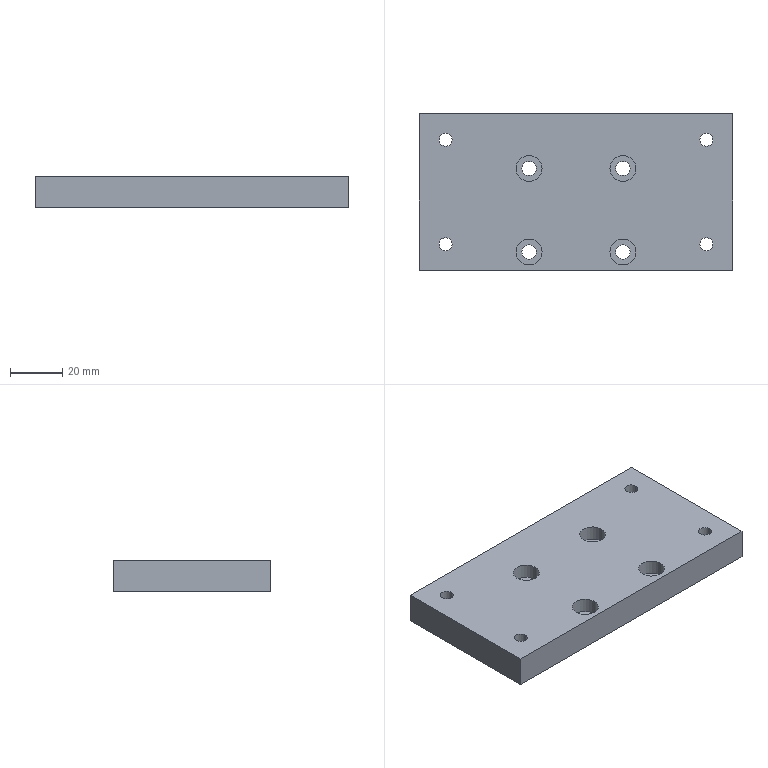Part | SolidWorks | features HoleWzd 2, 3DProfileFeature 1, Extrusion 1 | 1 solid | 34 faces | box 120 x 60 x 12 mm | volume 83068 mm3 | cylinder 24 | plane 10 | commonest cylinder face diameters 5 x8 5.5 x8 10 x8
STEP:
#1=CARTESIAN_POINT('',(-47.5,20.,0.));
#2=VERTEX_POINT('',#1);
#3=CARTESIAN_POINT('',(-52.5,20.,0.));
#4=VERTEX_POINT('',#3);
#5=CARTESIAN_POINT('',(-50.,20.,0.));
#6=DIRECTION('',(0.,0.,-1.));
#7=DIRECTION('',(-1.,0.,0.));
#8=AXIS2_PLACEMENT_3D('',#5,#6,#7);
#9=CIRCLE('',#8,2.5);
#10=EDGE_CURVE('',#2,#4,#9,.T.);
#11=ORIENTED_EDGE('',*,*,#10,.T.);
#12=CARTESIAN_POINT('',(-52.5,20.,12.));
#13=VERTEX_POINT('',#12);
#14=CARTESIAN_POINT('',(-52.5,20.,12.));
#15=DIRECTION('',(0.,0.,1.));
#16=VECTOR('',#15,1000.);
#17=LINE('',#14,#16);
#18=EDGE_CURVE('',#4,#13,#17,.T.);
#19=ORIENTED_EDGE('',*,*,#18,.T.);
#20=CARTESIAN_POINT('',(-47.5,20.,12.));
#21=VERTEX_POINT('',#20);
#22=CARTESIAN_POINT('',(-50.,20.,12.));
#23=DIRECTION('',(0.,0.,1.));
#24=DIRECTION('',(1.,0.,0.));
#25=AXIS2_PLACEMENT_3D('',#22,#23,#24);
#26=CIRCLE('',#25,2.5);
#27=EDGE_CURVE('',#13,#21,#26,.T.);
#28=ORIENTED_EDGE('',*,*,#27,.T.);
#29=CARTESIAN_POINT('',(-47.5,20.,12.));
#30=DIRECTION('',(0.,0.,1.));
#31=VECTOR('',#30,1000.);
#32=LINE('',#29,#31);
#33=EDGE_CURVE('',#2,#21,#32,.T.);
#34=ORIENTED_EDGE('',*,*,#33,.F.);
#35=EDGE_LOOP('',(#11,#19,#28,#34));
#36=FACE_OUTER_BOUND('',#35,.T.);
#37=CARTESIAN_POINT('',(-50.,20.,12.));
#38=DIRECTION('',(0.,0.,1.));
#39=DIRECTION('',(1.,0.,0.));
#40=AXIS2_PLACEMENT_3D('',#37,#38,#39);
#41=CYLINDRICAL_SURFACE('',#40,2.5);
#42=ADVANCED_FACE('',(#36),#41,.F.);
#43=CARTESIAN_POINT('',(-47.5,-20.,0.));
#44=VERTEX_POINT('',#43);
#45=CARTESIAN_POINT('',(-52.5,-20.,0.));
#46=VERTEX_POINT('',#45);
#47=CARTESIAN_POINT('',(-50.,-20.,0.));
#48=DIRECTION('',(0.,0.,-1.));
#49=DIRECTION('',(-1.,0.,0.));
#50=AXIS2_PLACEMENT_3D('',#47,#48,#49);
#51=CIRCLE('',#50,2.5);
#52=EDGE_CURVE('',#44,#46,#51,.T.);
#53=ORIENTED_EDGE('',*,*,#52,.T.);
#54=CARTESIAN_POINT('',(-52.5,-20.,12.));
#55=VERTEX_POINT('',#54);
#56=CARTESIAN_POINT('',(-52.5,-20.,12.));
#57=DIRECTION('',(0.,0.,1.));
#58=VECTOR('',#57,1000.);
#59=LINE('',#56,#58);
#60=EDGE_CURVE('',#46,#55,#59,.T.);
#61=ORIENTED_EDGE('',*,*,#60,.T.);
#62=CARTESIAN_POINT('',(-47.5,-20.,12.));
#63=VERTEX_POINT('',#62);
#64=CARTESIAN_POINT('',(-50.,-20.,12.));
#65=DIRECTION('',(0.,0.,1.));
#66=DIRECTION('',(1.,0.,0.));
#67=AXIS2_PLACEMENT_3D('',#64,#65,#66);
#68=CIRCLE('',#67,2.5);
#69=EDGE_CURVE('',#55,#63,#68,.T.);
#70=ORIENTED_EDGE('',*,*,#69,.T.);
#71=CARTESIAN_POINT('',(-47.5,-20.,12.));
#72=DIRECTION('',(0.,0.,1.));
#73=VECTOR('',#72,1000.);
#74=LINE('',#71,#73);
#75=EDGE_CURVE('',#44,#63,#74,.T.);
#76=ORIENTED_EDGE('',*,*,#75,.F.);
#77=EDGE_LOOP('',(#53,#61,#70,#76));
#78=FACE_OUTER_BOUND('',#77,.T.);
#79=CARTESIAN_POINT('',(-50.,-20.,12.));
#80=DIRECTION('',(0.,0.,1.));
#81=DIRECTION('',(1.,0.,0.));
#82=AXIS2_PLACEMENT_3D('',#79,#80,#81);
#83=CYLINDRICAL_SURFACE('',#82,2.5);
#84=ADVANCED_FACE('',(#78),#83,.F.);
#85=CARTESIAN_POINT('',(52.5,-20.,0.));
#86=VERTEX_POINT('',#85);
#87=CARTESIAN_POINT('',(47.5,-20.,0.));
#88=VERTEX_POINT('',#87);
#89=CARTESIAN_POINT('',(50.,-20.,0.));
#90=DIRECTION('',(0.,0.,-1.));
#91=DIRECTION('',(-1.,0.,0.));
#92=AXIS2_PLACEMENT_3D('',#89,#90,#91);
#93=CIRCLE('',#92,2.5);
#94=EDGE_CURVE('',#86,#88,#93,.T.);
#95=ORIENTED_EDGE('',*,*,#94,.T.);
#96=CARTESIAN_POINT('',(47.5,-20.,12.));
#97=VERTEX_POINT('',#96);
#98=CARTESIAN_POINT('',(47.5,-20.,12.));
#99=DIRECTION('',(0.,0.,1.));
#100=VECTOR('',#99,1000.);
#101=LINE('',#98,#100);
#102=EDGE_CURVE('',#88,#97,#101,.T.);
#103=ORIENTED_EDGE('',*,*,#102,.T.);
#104=CARTESIAN_POINT('',(52.5,-20.,12.));
#105=VERTEX_POINT('',#104);
#106=CARTESIAN_POINT('',(50.,-20.,12.));
#107=DIRECTION('',(0.,0.,1.));
#108=DIRECTION('',(1.,0.,0.));
#109=AXIS2_PLACEMENT_3D('',#106,#107,#108);
#110=CIRCLE('',#109,2.5);
#111=EDGE_CURVE('',#97,#105,#110,.T.);
#112=ORIENTED_EDGE('',*,*,#111,.T.);
#113=CARTESIAN_POINT('',(52.5,-20.,12.));
#114=DIRECTION('',(0.,0.,1.));
#115=VECTOR('',#114,1000.);
#116=LINE('',#113,#115);
#117=EDGE_CURVE('',#86,#105,#116,.T.);
#118=ORIENTED_EDGE('',*,*,#117,.F.);
#119=EDGE_LOOP('',(#95,#103,#112,#118));
#120=FACE_OUTER_BOUND('',#119,.T.);
#121=CARTESIAN_POINT('',(50.,-20.,12.));
#122=DIRECTION('',(0.,0.,1.));
#123=DIRECTION('',(1.,0.,0.));
#124=AXIS2_PLACEMENT_3D('',#121,#122,#123);
#125=CYLINDRICAL_SURFACE('',#124,2.5);
#126=ADVANCED_FACE('',(#120),#125,.F.);
#127=CARTESIAN_POINT('',(52.5,20.,0.));
#128=VERTEX_POINT('',#127);
#129=CARTESIAN_POINT('',(47.5,20.,0.));
#130=VERTEX_POINT('',#129);
#131=CARTESIAN_POINT('',(50.,20.,0.));
#132=DIRECTION('',(0.,0.,-1.));
#133=DIRECTION('',(-1.,0.,0.));
#134=AXIS2_PLACEMENT_3D('',#131,#132,#133);
#135=CIRCLE('',#134,2.5);
#136=EDGE_CURVE('',#128,#130,#135,.T.);
#137=ORIENTED_EDGE('',*,*,#136,.T.);
#138=CARTESIAN_POINT('',(47.5,20.,12.));
#139=VERTEX_POINT('',#138);
#140=CARTESIAN_POINT('',(47.5,20.,12.));
#141=DIRECTION('',(0.,0.,1.));
#142=VECTOR('',#141,1000.);
#143=LINE('',#140,#142);
#144=EDGE_CURVE('',#130,#139,#143,.T.);
#145=ORIENTED_EDGE('',*,*,#144,.T.);
#146=CARTESIAN_POINT('',(52.5,20.,12.));
#147=VERTEX_POINT('',#146);
#148=CARTESIAN_POINT('',(50.,20.,12.));
#149=DIRECTION('',(0.,0.,1.));
#150=DIRECTION('',(1.,0.,0.));
#151=AXIS2_PLACEMENT_3D('',#148,#149,#150);
#152=CIRCLE('',#151,2.5);
#153=EDGE_CURVE('',#139,#147,#152,.T.);
#154=ORIENTED_EDGE('',*,*,#153,.T.);
#155=CARTESIAN_POINT('',(52.5,20.,12.));
#156=DIRECTION('',(0.,0.,1.));
#157=VECTOR('',#156,1000.);
#158=LINE('',#155,#157);
#159=EDGE_CURVE('',#128,#147,#158,.T.);
#160=ORIENTED_EDGE('',*,*,#159,.F.);
#161=EDGE_LOOP('',(#137,#145,#154,#160));
#162=FACE_OUTER_BOUND('',#161,.T.);
#163=CARTESIAN_POINT('',(50.,20.,12.));
#164=DIRECTION('',(0.,0.,1.));
#165=DIRECTION('',(1.,0.,0.));
#166=AXIS2_PLACEMENT_3D('',#163,#164,#165);
#167=CYLINDRICAL_SURFACE('',#166,2.5);
#168=ADVANCED_FACE('',(#162),#167,.F.);
#169=CARTESIAN_POINT('',(-23.,9.,6.3));
#170=VERTEX_POINT('',#169);
#171=CARTESIAN_POINT('',(-13.,9.,6.3));
#172=VERTEX_POINT('',#171);
#173=CARTESIAN_POINT('',(-18.,9.,6.3));
#174=DIRECTION('',(0.,0.,1.));
#175=DIRECTION('',(1.,0.,0.));
#176=AXIS2_PLACEMENT_3D('',#173,#174,#175);
#177=CIRCLE('',#176,5.);
#178=EDGE_CURVE('',#170,#172,#177,.T.);
#179=ORIENTED_EDGE('',*,*,#178,.F.);
#180=CARTESIAN_POINT('',(-23.,9.,12.));
#181=VERTEX_POINT('',#180);
#182=CARTESIAN_POINT('',(-23.,9.,12.));
#183=DIRECTION('',(0.,0.,1.));
#184=VECTOR('',#183,1000.);
#185=LINE('',#182,#184);
#186=EDGE_CURVE('',#170,#181,#185,.T.);
#187=ORIENTED_EDGE('',*,*,#186,.T.);
#188=CARTESIAN_POINT('',(-13.,9.,12.));
#189=VERTEX_POINT('',#188);
#190=CARTESIAN_POINT('',(-18.,9.,12.));
#191=DIRECTION('',(0.,0.,1.));
#192=DIRECTION('',(1.,0.,0.));
#193=AXIS2_PLACEMENT_3D('',#190,#191,#192);
#194=CIRCLE('',#193,5.);
#195=EDGE_CURVE('',#181,#189,#194,.T.);
#196=ORIENTED_EDGE('',*,*,#195,.T.);
#197=CARTESIAN_POINT('',(-13.,9.,12.));
#198=DIRECTION('',(0.,0.,1.));
#199=VECTOR('',#198,1000.);
#200=LINE('',#197,#199);
#201=EDGE_CURVE('',#172,#189,#200,.T.);
#202=ORIENTED_EDGE('',*,*,#201,.F.);
#203=EDGE_LOOP('',(#179,#187,#196,#202));
#204=FACE_OUTER_BOUND('',#203,.T.);
#205=CARTESIAN_POINT('',(-18.,9.,12.));
#206=DIRECTION('',(0.,0.,1.));
#207=DIRECTION('',(1.,0.,0.));
#208=AXIS2_PLACEMENT_3D('',#205,#206,#207);
#209=CYLINDRICAL_SURFACE('',#208,5.);
#210=ADVANCED_FACE('',(#204),#209,.F.);
#211=CARTESIAN_POINT('',(-15.25,9.,0.));
#212=VERTEX_POINT('',#211);
#213=CARTESIAN_POINT('',(-20.75,9.,0.));
#214=VERTEX_POINT('',#213);
#215=CARTESIAN_POINT('',(-18.,9.,0.));
#216=DIRECTION('',(0.,0.,-1.));
#217=DIRECTION('',(-1.,0.,0.));
#218=AXIS2_PLACEMENT_3D('',#215,#216,#217);
#219=CIRCLE('',#218,2.75);
#220=EDGE_CURVE('',#212,#214,#219,.T.);
#221=ORIENTED_EDGE('',*,*,#220,.T.);
#222=CARTESIAN_POINT('',(-20.75,9.,6.3));
#223=VERTEX_POINT('',#222);
#224=CARTESIAN_POINT('',(-20.75,9.,12.));
#225=DIRECTION('',(0.,0.,1.));
#226=VECTOR('',#225,1000.);
#227=LINE('',#224,#226);
#228=EDGE_CURVE('',#214,#223,#227,.T.);
#229=ORIENTED_EDGE('',*,*,#228,.T.);
#230=CARTESIAN_POINT('',(-15.25,9.,6.3));
#231=VERTEX_POINT('',#230);
#232=CARTESIAN_POINT('',(-18.,9.,6.3));
#233=DIRECTION('',(0.,0.,1.));
#234=DIRECTION('',(1.,0.,0.));
#235=AXIS2_PLACEMENT_3D('',#232,#233,#234);
#236=CIRCLE('',#235,2.75);
#237=EDGE_CURVE('',#223,#231,#236,.T.);
#238=ORIENTED_EDGE('',*,*,#237,.T.);
#239=CARTESIAN_POINT('',(-15.25,9.,12.));
#240=DIRECTION('',(0.,0.,1.));
#241=VECTOR('',#240,1000.);
#242=LINE('',#239,#241);
#243=EDGE_CURVE('',#212,#231,#242,.T.);
#244=ORIENTED_EDGE('',*,*,#243,.F.);
#245=EDGE_LOOP('',(#221,#229,#238,#244));
#246=FACE_OUTER_BOUND('',#245,.T.);
#247=CARTESIAN_POINT('',(-18.,9.,12.));
#248=DIRECTION('',(0.,0.,1.));
#249=DIRECTION('',(1.,0.,0.));
#250=AXIS2_PLACEMENT_3D('',#247,#248,#249);
#251=CYLINDRICAL_SURFACE('',#250,2.75);
#252=ADVANCED_FACE('',(#246),#251,.F.);
#253=CARTESIAN_POINT('',(13.,9.,6.3));
#254=VERTEX_POINT('',#253);
#255=CARTESIAN_POINT('',(23.,9.,6.3));
#256=VERTEX_POINT('',#255);
#257=CARTESIAN_POINT('',(18.,9.,6.3));
#258=DIRECTION('',(0.,0.,1.));
#259=DIRECTION('',(1.,0.,0.));
#260=AXIS2_PLACEMENT_3D('',#257,#258,#259);
#261=CIRCLE('',#260,5.);
#262=EDGE_CURVE('',#254,#256,#261,.T.);
#263=ORIENTED_EDGE('',*,*,#262,.F.);
#264=CARTESIAN_POINT('',(13.,9.,12.));
#265=VERTEX_POINT('',#264);
#266=CARTESIAN_POINT('',(13.,9.,12.));
#267=DIRECTION('',(0.,0.,1.));
#268=VECTOR('',#267,1000.);
#269=LINE('',#266,#268);
#270=EDGE_CURVE('',#254,#265,#269,.T.);
#271=ORIENTED_EDGE('',*,*,#270,.T.);
#272=CARTESIAN_POINT('',(23.,9.,12.));
#273=VERTEX_POINT('',#272);
#274=CARTESIAN_POINT('',(18.,9.,12.));
#275=DIRECTION('',(0.,0.,1.));
#276=DIRECTION('',(1.,0.,0.));
#277=AXIS2_PLACEMENT_3D('',#274,#275,#276);
#278=CIRCLE('',#277,5.);
#279=EDGE_CURVE('',#265,#273,#278,.T.);
#280=ORIENTED_EDGE('',*,*,#279,.T.);
#281=CARTESIAN_POINT('',(23.,9.,12.));
#282=DIRECTION('',(0.,0.,1.));
#283=VECTOR('',#282,1000.);
#284=LINE('',#281,#283);
#285=EDGE_CURVE('',#256,#273,#284,.T.);
#286=ORIENTED_EDGE('',*,*,#285,.F.);
#287=EDGE_LOOP('',(#263,#271,#280,#286));
#288=FACE_OUTER_BOUND('',#287,.T.);
#289=CARTESIAN_POINT('',(18.,9.,12.));
#290=DIRECTION('',(0.,0.,1.));
#291=DIRECTION('',(1.,0.,0.));
#292=AXIS2_PLACEMENT_3D('',#289,#290,#291);
#293=CYLINDRICAL_SURFACE('',#292,5.);
#294=ADVANCED_FACE('',(#288),#293,.F.);
#295=CARTESIAN_POINT('',(20.75,9.,0.));
#296=VERTEX_POINT('',#295);
#297=CARTESIAN_POINT('',(15.25,9.,0.));
#298=VERTEX_POINT('',#297);
#299=CARTESIAN_POINT('',(18.,9.,0.));
#300=DIRECTION('',(0.,0.,-1.));
#301=DIRECTION('',(-1.,0.,0.));
#302=AXIS2_PLACEMENT_3D('',#299,#300,#301);
#303=CIRCLE('',#302,2.75);
#304=EDGE_CURVE('',#296,#298,#303,.T.);
#305=ORIENTED_EDGE('',*,*,#304,.T.);
#306=CARTESIAN_POINT('',(15.25,9.,6.3));
#307=VERTEX_POINT('',#306);
#308=CARTESIAN_POINT('',(15.25,9.,12.));
#309=DIRECTION('',(0.,0.,1.));
#310=VECTOR('',#309,1000.);
#311=LINE('',#308,#310);
#312=EDGE_CURVE('',#298,#307,#311,.T.);
#313=ORIENTED_EDGE('',*,*,#312,.T.);
#314=CARTESIAN_POINT('',(20.75,9.,6.3));
#315=VERTEX_POINT('',#314);
#316=CARTESIAN_POINT('',(18.,9.,6.3));
#317=DIRECTION('',(0.,0.,1.));
#318=DIRECTION('',(1.,0.,0.));
#319=AXIS2_PLACEMENT_3D('',#316,#317,#318);
#320=CIRCLE('',#319,2.75);
#321=EDGE_CURVE('',#307,#315,#320,.T.);
#322=ORIENTED_EDGE('',*,*,#321,.T.);
#323=CARTESIAN_POINT('',(20.75,9.,12.));
#324=DIRECTION('',(0.,0.,1.));
#325=VECTOR('',#324,1000.);
#326=LINE('',#323,#325);
#327=EDGE_CURVE('',#296,#315,#326,.T.);
#328=ORIENTED_EDGE('',*,*,#327,.F.);
#329=EDGE_LOOP('',(#305,#313,#322,#328));
#330=FACE_OUTER_BOUND('',#329,.T.);
#331=CARTESIAN_POINT('',(18.,9.,12.));
#332=DIRECTION('',(0.,0.,1.));
#333=DIRECTION('',(1.,0.,0.));
#334=AXIS2_PLACEMENT_3D('',#331,#332,#333);
#335=CYLINDRICAL_SURFACE('',#334,2.75);
#336=ADVANCED_FACE('',(#330),#335,.F.);
#337=CARTESIAN_POINT('',(-23.,-23.,6.3));
#338=VERTEX_POINT('',#337);
#339=CARTESIAN_POINT('',(-13.,-23.,6.3));
#340=VERTEX_POINT('',#339);
#341=CARTESIAN_POINT('',(-18.,-23.,6.3));
#342=DIRECTION('',(0.,0.,1.));
#343=DIRECTION('',(1.,0.,0.));
#344=AXIS2_PLACEMENT_3D('',#341,#342,#343);
#345=CIRCLE('',#344,5.);
#346=EDGE_CURVE('',#338,#340,#345,.T.);
#347=ORIENTED_EDGE('',*,*,#346,.F.);
#348=CARTESIAN_POINT('',(-23.,-23.,12.));
#349=VERTEX_POINT('',#348);
#350=CARTESIAN_POINT('',(-23.,-23.,12.));
#351=DIRECTION('',(0.,0.,1.));
#352=VECTOR('',#351,1000.);
#353=LINE('',#350,#352);
#354=EDGE_CURVE('',#338,#349,#353,.T.);
#355=ORIENTED_EDGE('',*,*,#354,.T.);
#356=CARTESIAN_POINT('',(-13.,-23.,12.));
#357=VERTEX_POINT('',#356);
#358=CARTESIAN_POINT('',(-18.,-23.,12.));
#359=DIRECTION('',(0.,0.,1.));
#360=DIRECTION('',(1.,0.,0.));
#361=AXIS2_PLACEMENT_3D('',#358,#359,#360);
#362=CIRCLE('',#361,5.);
#363=EDGE_CURVE('',#349,#357,#362,.T.);
#364=ORIENTED_EDGE('',*,*,#363,.T.);
#365=CARTESIAN_POINT('',(-13.,-23.,12.));
#366=DIRECTION('',(0.,0.,1.));
#367=VECTOR('',#366,1000.);
#368=LINE('',#365,#367);
#369=EDGE_CURVE('',#340,#357,#368,.T.);
#370=ORIENTED_EDGE('',*,*,#369,.F.);
#371=EDGE_LOOP('',(#347,#355,#364,#370));
#372=FACE_OUTER_BOUND('',#371,.T.);
#373=CARTESIAN_POINT('',(-18.,-23.,12.));
#374=DIRECTION('',(0.,0.,1.));
#375=DIRECTION('',(1.,0.,0.));
#376=AXIS2_PLACEMENT_3D('',#373,#374,#375);
#377=CYLINDRICAL_SURFACE('',#376,5.);
#378=ADVANCED_FACE('',(#372),#377,.F.);
#379=CARTESIAN_POINT('',(-15.25,-23.,0.));
#380=VERTEX_POINT('',#379);
#381=CARTESIAN_POINT('',(-20.75,-23.,0.));
#382=VERTEX_POINT('',#381);
#383=CARTESIAN_POINT('',(-18.,-23.,0.));
#384=DIRECTION('',(0.,0.,-1.));
#385=DIRECTION('',(-1.,0.,0.));
#386=AXIS2_PLACEMENT_3D('',#383,#384,#385);
#387=CIRCLE('',#386,2.75);
#388=EDGE_CURVE('',#380,#382,#387,.T.);
#389=ORIENTED_EDGE('',*,*,#388,.T.);
#390=CARTESIAN_POINT('',(-20.75,-23.,6.3));
#391=VERTEX_POINT('',#390);
#392=CARTESIAN_POINT('',(-20.75,-23.,12.));
#393=DIRECTION('',(0.,0.,1.));
#394=VECTOR('',#393,1000.);
#395=LINE('',#392,#394);
#396=EDGE_CURVE('',#382,#391,#395,.T.);
#397=ORIENTED_EDGE('',*,*,#396,.T.);
#398=CARTESIAN_POINT('',(-15.25,-23.,6.3));
#399=VERTEX_POINT('',#398);
#400=CARTESIAN_POINT('',(-18.,-23.,6.3));
#401=DIRECTION('',(0.,0.,1.));
#402=DIRECTION('',(1.,0.,0.));
#403=AXIS2_PLACEMENT_3D('',#400,#401,#402);
#404=CIRCLE('',#403,2.75);
#405=EDGE_CURVE('',#391,#399,#404,.T.);
#406=ORIENTED_EDGE('',*,*,#405,.T.);
#407=CARTESIAN_POINT('',(-15.25,-23.,12.));
#408=DIRECTION('',(0.,0.,1.));
#409=VECTOR('',#408,1000.);
#410=LINE('',#407,#409);
#411=EDGE_CURVE('',#380,#399,#410,.T.);
#412=ORIENTED_EDGE('',*,*,#411,.F.);
#413=EDGE_LOOP('',(#389,#397,#406,#412));
#414=FACE_OUTER_BOUND('',#413,.T.);
#415=CARTESIAN_POINT('',(-18.,-23.,12.));
#416=DIRECTION('',(0.,0.,1.));
#417=DIRECTION('',(1.,0.,0.));
#418=AXIS2_PLACEMENT_3D('',#415,#416,#417);
#419=CYLINDRICAL_SURFACE('',#418,2.75);
#420=ADVANCED_FACE('',(#414),#419,.F.);
#421=CARTESIAN_POINT('',(13.,-23.,6.3));
#422=VERTEX_POINT('',#421);
#423=CARTESIAN_POINT('',(23.,-23.,6.3));
#424=VERTEX_POINT('',#423);
#425=CARTESIAN_POINT('',(18.,-23.,6.3));
#426=DIRECTION('',(0.,0.,1.));
#427=DIRECTION('',(1.,0.,0.));
#428=AXIS2_PLACEMENT_3D('',#425,#426,#427);
#429=CIRCLE('',#428,5.);
#430=EDGE_CURVE('',#422,#424,#429,.T.);
#431=ORIENTED_EDGE('',*,*,#430,.F.);
#432=CARTESIAN_POINT('',(13.,-23.,12.));
#433=VERTEX_POINT('',#432);
#434=CARTESIAN_POINT('',(13.,-23.,12.));
#435=DIRECTION('',(0.,0.,1.));
#436=VECTOR('',#435,1000.);
#437=LINE('',#434,#436);
#438=EDGE_CURVE('',#422,#433,#437,.T.);
#439=ORIENTED_EDGE('',*,*,#438,.T.);
#440=CARTESIAN_POINT('',(23.,-23.,12.));
#441=VERTEX_POINT('',#440);
#442=CARTESIAN_POINT('',(18.,-23.,12.));
#443=DIRECTION('',(0.,0.,1.));
#444=DIRECTION('',(1.,0.,0.));
#445=AXIS2_PLACEMENT_3D('',#442,#443,#444);
#446=CIRCLE('',#445,5.);
#447=EDGE_CURVE('',#433,#441,#446,.T.);
#448=ORIENTED_EDGE('',*,*,#447,.T.);
#449=CARTESIAN_POINT('',(23.,-23.,12.));
#450=DIRECTION('',(0.,0.,1.));
#451=VECTOR('',#450,1000.);
#452=LINE('',#449,#451);
#453=EDGE_CURVE('',#424,#441,#452,.T.);
#454=ORIENTED_EDGE('',*,*,#453,.F.);
#455=EDGE_LOOP('',(#431,#439,#448,#454));
#456=FACE_OUTER_BOUND('',#455,.T.);
#457=CARTESIAN_POINT('',(18.,-23.,12.));
#458=DIRECTION('',(0.,0.,1.));
#459=DIRECTION('',(1.,0.,0.));
#460=AXIS2_PLACEMENT_3D('',#457,#458,#459);
#461=CYLINDRICAL_SURFACE('',#460,5.);
#462=ADVANCED_FACE('',(#456),#461,.F.);
#463=CARTESIAN_POINT('',(20.75,-23.,0.));
#464=VERTEX_POINT('',#463);
#465=CARTESIAN_POINT('',(15.25,-23.,0.));
#466=VERTEX_POINT('',#465);
#467=CARTESIAN_POINT('',(18.,-23.,0.));
#468=DIRECTION('',(0.,0.,-1.));
#469=DIRECTION('',(-1.,0.,0.));
#470=AXIS2_PLACEMENT_3D('',#467,#468,#469);
#471=CIRCLE('',#470,2.75);
#472=EDGE_CURVE('',#464,#466,#471,.T.);
#473=ORIENTED_EDGE('',*,*,#472,.T.);
#474=CARTESIAN_POINT('',(15.25,-23.,6.3));
#475=VERTEX_POINT('',#474);
#476=CARTESIAN_POINT('',(15.25,-23.,12.));
#477=DIRECTION('',(0.,0.,1.));
#478=VECTOR('',#477,1000.);
#479=LINE('',#476,#478);
#480=EDGE_CURVE('',#466,#475,#479,.T.);
#481=ORIENTED_EDGE('',*,*,#480,.T.);
#482=CARTESIAN_POINT('',(20.75,-23.,6.3));
#483=VERTEX_POINT('',#482);
#484=CARTESIAN_POINT('',(18.,-23.,6.3));
#485=DIRECTION('',(0.,0.,1.));
#486=DIRECTION('',(1.,0.,0.));
#487=AXIS2_PLACEMENT_3D('',#484,#485,#486);
#488=CIRCLE('',#487,2.75);
#489=EDGE_CURVE('',#475,#483,#488,.T.);
#490=ORIENTED_EDGE('',*,*,#489,.T.);
#491=CARTESIAN_POINT('',(20.75,-23.,12.));
#492=DIRECTION('',(0.,0.,1.));
#493=VECTOR('',#492,1000.);
#494=LINE('',#491,#493);
#495=EDGE_CURVE('',#464,#483,#494,.T.);
#496=ORIENTED_EDGE('',*,*,#495,.F.);
#497=EDGE_LOOP('',(#473,#481,#490,#496));
#498=FACE_OUTER_BOUND('',#497,.T.);
#499=CARTESIAN_POINT('',(18.,-23.,12.));
#500=DIRECTION('',(0.,0.,1.));
#501=DIRECTION('',(1.,0.,0.));
#502=AXIS2_PLACEMENT_3D('',#499,#500,#501);
#503=CYLINDRICAL_SURFACE('',#502,2.75);
#504=ADVANCED_FACE('',(#498),#503,.F.);
#505=CARTESIAN_POINT('',(-50.,20.,12.));
#506=DIRECTION('',(0.,0.,1.));
#507=DIRECTION('',(1.,0.,0.));
#508=AXIS2_PLACEMENT_3D('',#505,#506,#507);
#509=CIRCLE('',#508,2.5);
#510=EDGE_CURVE('',#21,#13,#509,.T.);
#511=ORIENTED_EDGE('',*,*,#510,.F.);
#512=ORIENTED_EDGE('',*,*,#27,.F.);
#513=EDGE_LOOP('',(#511,#512));
#514=FACE_BOUND('',#513,.T.);
#515=CARTESIAN_POINT('',(-50.,-20.,12.));
#516=DIRECTION('',(0.,0.,1.));
#517=DIRECTION('',(1.,0.,0.));
#518=AXIS2_PLACEMENT_3D('',#515,#516,#517);
#519=CIRCLE('',#518,2.5);
#520=EDGE_CURVE('',#63,#55,#519,.T.);
#521=ORIENTED_EDGE('',*,*,#520,.F.);
#522=ORIENTED_EDGE('',*,*,#69,.F.);
#523=EDGE_LOOP('',(#521,#522));
#524=FACE_BOUND('',#523,.T.);
#525=CARTESIAN_POINT('',(50.,-20.,12.));
#526=DIRECTION('',(0.,0.,1.));
#527=DIRECTION('',(1.,0.,0.));
#528=AXIS2_PLACEMENT_3D('',#525,#526,#527);
#529=CIRCLE('',#528,2.5);
#530=EDGE_CURVE('',#105,#97,#529,.T.);
#531=ORIENTED_EDGE('',*,*,#530,.F.);
#532=ORIENTED_EDGE('',*,*,#111,.F.);
#533=EDGE_LOOP('',(#531,#532));
#534=FACE_BOUND('',#533,.T.);
#535=CARTESIAN_POINT('',(50.,20.,12.));
#536=DIRECTION('',(0.,0.,1.));
#537=DIRECTION('',(1.,0.,0.));
#538=AXIS2_PLACEMENT_3D('',#535,#536,#537);
#539=CIRCLE('',#538,2.5);
#540=EDGE_CURVE('',#147,#139,#539,.T.);
#541=ORIENTED_EDGE('',*,*,#540,.F.);
#542=ORIENTED_EDGE('',*,*,#153,.F.);
#543=EDGE_LOOP('',(#541,#542));
#544=FACE_BOUND('',#543,.T.);
#545=CARTESIAN_POINT('',(-18.,9.,12.));
#546=DIRECTION('',(0.,0.,1.));
#547=DIRECTION('',(1.,0.,0.));
#548=AXIS2_PLACEMENT_3D('',#545,#546,#547);
#549=CIRCLE('',#548,5.);
#550=EDGE_CURVE('',#189,#181,#549,.T.);
#551=ORIENTED_EDGE('',*,*,#550,.F.);
#552=ORIENTED_EDGE('',*,*,#195,.F.);
#553=EDGE_LOOP('',(#551,#552));
#554=FACE_BOUND('',#553,.T.);
#555=CARTESIAN_POINT('',(18.,9.,12.));
#556=DIRECTION('',(0.,0.,1.));
#557=DIRECTION('',(1.,0.,0.));
#558=AXIS2_PLACEMENT_3D('',#555,#556,#557);
#559=CIRCLE('',#558,5.);
#560=EDGE_CURVE('',#273,#265,#559,.T.);
#561=ORIENTED_EDGE('',*,*,#560,.F.);
#562=ORIENTED_EDGE('',*,*,#279,.F.);
#563=EDGE_LOOP('',(#561,#562));
#564=FACE_BOUND('',#563,.T.);
#565=CARTESIAN_POINT('',(-18.,-23.,12.));
#566=DIRECTION('',(0.,0.,1.));
#567=DIRECTION('',(1.,0.,0.));
#568=AXIS2_PLACEMENT_3D('',#565,#566,#567);
#569=CIRCLE('',#568,5.);
#570=EDGE_CURVE('',#357,#349,#569,.T.);
#571=ORIENTED_EDGE('',*,*,#570,.F.);
#572=ORIENTED_EDGE('',*,*,#363,.F.);
#573=EDGE_LOOP('',(#571,#572));
#574=FACE_BOUND('',#573,.T.);
#575=CARTESIAN_POINT('',(18.,-23.,12.));
#576=DIRECTION('',(0.,0.,1.));
#577=DIRECTION('',(1.,0.,0.));
#578=AXIS2_PLACEMENT_3D('',#575,#576,#577);
#579=CIRCLE('',#578,5.);
#580=EDGE_CURVE('',#441,#433,#579,.T.);
#581=ORIENTED_EDGE('',*,*,#580,.F.);
#582=ORIENTED_EDGE('',*,*,#447,.F.);
#583=EDGE_LOOP('',(#581,#582));
#584=FACE_BOUND('',#583,.T.);
#585=CARTESIAN_POINT('',(60.,-30.,12.));
#586=VERTEX_POINT('',#585);
#587=CARTESIAN_POINT('',(60.,30.,12.));
#588=VERTEX_POINT('',#587);
#589=CARTESIAN_POINT('',(60.,-30.,12.));
#590=DIRECTION('',(0.,1.,0.));
#591=VECTOR('',#590,1000.);
#592=LINE('',#589,#591);
#593=EDGE_CURVE('',#586,#588,#592,.T.);
#594=ORIENTED_EDGE('',*,*,#593,.T.);
#595=CARTESIAN_POINT('',(-60.,30.,12.));
#596=VERTEX_POINT('',#595);
#597=CARTESIAN_POINT('',(-60.,30.,12.));
#598=DIRECTION('',(-1.,0.,0.));
#599=VECTOR('',#598,1000.);
#600=LINE('',#597,#599);
#601=EDGE_CURVE('',#588,#596,#600,.T.);
#602=ORIENTED_EDGE('',*,*,#601,.T.);
#603=CARTESIAN_POINT('',(-60.,-30.,12.));
#604=VERTEX_POINT('',#603);
#605=CARTESIAN_POINT('',(-60.,-30.,12.));
#606=DIRECTION('',(0.,-1.,0.));
#607=VECTOR('',#606,1000.);
#608=LINE('',#605,#607);
#609=EDGE_CURVE('',#596,#604,#608,.T.);
#610=ORIENTED_EDGE('',*,*,#609,.T.);
#611=CARTESIAN_POINT('',(-60.,-30.,12.));
#612=DIRECTION('',(1.,0.,0.));
#613=VECTOR('',#612,1000.);
#614=LINE('',#611,#613);
#615=EDGE_CURVE('',#604,#586,#614,.T.);
#616=ORIENTED_EDGE('',*,*,#615,.T.);
#617=EDGE_LOOP('',(#594,#602,#610,#616));
#618=FACE_OUTER_BOUND('',#617,.T.);
#619=CARTESIAN_POINT('',(0.,0.,12.));
#620=DIRECTION('',(0.,0.,-1.));
#621=DIRECTION('',(-1.,0.,0.));
#622=AXIS2_PLACEMENT_3D('',#619,#620,#621);
#623=PLANE('',#622);
#624=ADVANCED_FACE('',(#514,#524,#534,#544,#554,#564,#574,#584,#618),#623,.F.);
#625=ORIENTED_EDGE('',*,*,#10,.F.);
#626=CARTESIAN_POINT('',(-50.,20.,0.));
#627=DIRECTION('',(0.,0.,-1.));
#628=DIRECTION('',(-1.,0.,0.));
#629=AXIS2_PLACEMENT_3D('',#626,#627,#628);
#630=CIRCLE('',#629,2.5);
#631=EDGE_CURVE('',#4,#2,#630,.T.);
#632=ORIENTED_EDGE('',*,*,#631,.F.);
#633=EDGE_LOOP('',(#625,#632));
#634=FACE_BOUND('',#633,.T.);
#635=ORIENTED_EDGE('',*,*,#52,.F.);
#636=CARTESIAN_POINT('',(-50.,-20.,0.));
#637=DIRECTION('',(0.,0.,-1.));
#638=DIRECTION('',(-1.,0.,0.));
#639=AXIS2_PLACEMENT_3D('',#636,#637,#638);
#640=CIRCLE('',#639,2.5);
#641=EDGE_CURVE('',#46,#44,#640,.T.);
#642=ORIENTED_EDGE('',*,*,#641,.F.);
#643=EDGE_LOOP('',(#635,#642));
#644=FACE_BOUND('',#643,.T.);
#645=ORIENTED_EDGE('',*,*,#94,.F.);
#646=CARTESIAN_POINT('',(50.,-20.,0.));
#647=DIRECTION('',(0.,0.,-1.));
#648=DIRECTION('',(-1.,0.,0.));
#649=AXIS2_PLACEMENT_3D('',#646,#647,#648);
#650=CIRCLE('',#649,2.5);
#651=EDGE_CURVE('',#88,#86,#650,.T.);
#652=ORIENTED_EDGE('',*,*,#651,.F.);
#653=EDGE_LOOP('',(#645,#652));
#654=FACE_BOUND('',#653,.T.);
#655=ORIENTED_EDGE('',*,*,#136,.F.);
#656=CARTESIAN_POINT('',(50.,20.,0.));
#657=DIRECTION('',(0.,0.,-1.));
#658=DIRECTION('',(-1.,0.,0.));
#659=AXIS2_PLACEMENT_3D('',#656,#657,#658);
#660=CIRCLE('',#659,2.5);
#661=EDGE_CURVE('',#130,#128,#660,.T.);
#662=ORIENTED_EDGE('',*,*,#661,.F.);
#663=EDGE_LOOP('',(#655,#662));
#664=FACE_BOUND('',#663,.T.);
#665=ORIENTED_EDGE('',*,*,#220,.F.);
#666=CARTESIAN_POINT('',(-18.,9.,0.));
#667=DIRECTION('',(0.,0.,-1.));
#668=DIRECTION('',(-1.,0.,0.));
#669=AXIS2_PLACEMENT_3D('',#666,#667,#668);
#670=CIRCLE('',#669,2.75);
#671=EDGE_CURVE('',#214,#212,#670,.T.);
#672=ORIENTED_EDGE('',*,*,#671,.F.);
#673=EDGE_LOOP('',(#665,#672));
#674=FACE_BOUND('',#673,.T.);
#675=ORIENTED_EDGE('',*,*,#304,.F.);
#676=CARTESIAN_POINT('',(18.,9.,0.));
#677=DIRECTION('',(0.,0.,-1.));
#678=DIRECTION('',(-1.,0.,0.));
#679=AXIS2_PLACEMENT_3D('',#676,#677,#678);
#680=CIRCLE('',#679,2.75);
#681=EDGE_CURVE('',#298,#296,#680,.T.);
#682=ORIENTED_EDGE('',*,*,#681,.F.);
#683=EDGE_LOOP('',(#675,#682));
#684=FACE_BOUND('',#683,.T.);
#685=ORIENTED_EDGE('',*,*,#388,.F.);
#686=CARTESIAN_POINT('',(-18.,-23.,0.));
#687=DIRECTION('',(0.,0.,-1.));
#688=DIRECTION('',(-1.,0.,0.));
#689=AXIS2_PLACEMENT_3D('',#686,#687,#688);
#690=CIRCLE('',#689,2.75);
#691=EDGE_CURVE('',#382,#380,#690,.T.);
#692=ORIENTED_EDGE('',*,*,#691,.F.);
#693=EDGE_LOOP('',(#685,#692));
#694=FACE_BOUND('',#693,.T.);
#695=ORIENTED_EDGE('',*,*,#472,.F.);
#696=CARTESIAN_POINT('',(18.,-23.,0.));
#697=DIRECTION('',(0.,0.,-1.));
#698=DIRECTION('',(-1.,0.,0.));
#699=AXIS2_PLACEMENT_3D('',#696,#697,#698);
#700=CIRCLE('',#699,2.75);
#701=EDGE_CURVE('',#466,#464,#700,.T.);
#702=ORIENTED_EDGE('',*,*,#701,.F.);
#703=EDGE_LOOP('',(#695,#702));
#704=FACE_BOUND('',#703,.T.);
#705=CARTESIAN_POINT('',(60.,-30.,0.));
#706=VERTEX_POINT('',#705);
#707=CARTESIAN_POINT('',(60.,30.,0.));
#708=VERTEX_POINT('',#707);
#709=CARTESIAN_POINT('',(60.,-30.,0.));
#710=DIRECTION('',(0.,1.,0.));
#711=VECTOR('',#710,1000.);
#712=LINE('',#709,#711);
#713=EDGE_CURVE('',#706,#708,#712,.T.);
#714=ORIENTED_EDGE('',*,*,#713,.F.);
#715=CARTESIAN_POINT('',(-60.,-30.,0.));
#716=VERTEX_POINT('',#715);
#717=CARTESIAN_POINT('',(-60.,-30.,0.));
#718=DIRECTION('',(1.,0.,0.));
#719=VECTOR('',#718,1000.);
#720=LINE('',#717,#719);
#721=EDGE_CURVE('',#716,#706,#720,.T.);
#722=ORIENTED_EDGE('',*,*,#721,.F.);
#723=CARTESIAN_POINT('',(-60.,30.,0.));
#724=VERTEX_POINT('',#723);
#725=CARTESIAN_POINT('',(-60.,-30.,0.));
#726=DIRECTION('',(0.,-1.,0.));
#727=VECTOR('',#726,1000.);
#728=LINE('',#725,#727);
#729=EDGE_CURVE('',#724,#716,#728,.T.);
#730=ORIENTED_EDGE('',*,*,#729,.F.);
#731=CARTESIAN_POINT('',(-60.,30.,0.));
#732=DIRECTION('',(-1.,0.,0.));
#733=VECTOR('',#732,1000.);
#734=LINE('',#731,#733);
#735=EDGE_CURVE('',#708,#724,#734,.T.);
#736=ORIENTED_EDGE('',*,*,#735,.F.);
#737=EDGE_LOOP('',(#714,#722,#730,#736));
#738=FACE_OUTER_BOUND('',#737,.T.);
#739=CARTESIAN_POINT('',(0.,0.,0.));
#740=DIRECTION('',(0.,0.,-1.));
#741=DIRECTION('',(-1.,0.,0.));
#742=AXIS2_PLACEMENT_3D('',#739,#740,#741);
#743=PLANE('',#742);
#744=ADVANCED_FACE('',(#634,#644,#654,#664,#674,#684,#694,#704,#738),#743,.T.);
#745=ORIENTED_EDGE('',*,*,#713,.T.);
#746=CARTESIAN_POINT('',(60.,30.,12.));
#747=DIRECTION('',(0.,0.,-1.));
#748=VECTOR('',#747,1000.);
#749=LINE('',#746,#748);
#750=EDGE_CURVE('',#588,#708,#749,.T.);
#751=ORIENTED_EDGE('',*,*,#750,.F.);
#752=ORIENTED_EDGE('',*,*,#593,.F.);
#753=CARTESIAN_POINT('',(60.,-30.,12.));
#754=DIRECTION('',(0.,0.,-1.));
#755=VECTOR('',#754,1000.);
#756=LINE('',#753,#755);
#757=EDGE_CURVE('',#586,#706,#756,.T.);
#758=ORIENTED_EDGE('',*,*,#757,.T.);
#759=EDGE_LOOP('',(#745,#751,#752,#758));
#760=FACE_OUTER_BOUND('',#759,.T.);
#761=CARTESIAN_POINT('',(60.,-30.,12.));
#762=DIRECTION('',(-1.,0.,0.));
#763=DIRECTION('',(0.,0.,1.));
#764=AXIS2_PLACEMENT_3D('',#761,#762,#763);
#765=PLANE('',#764);
#766=ADVANCED_FACE('',(#760),#765,.F.);
#767=ORIENTED_EDGE('',*,*,#735,.T.);
#768=CARTESIAN_POINT('',(-60.,30.,12.));
#769=DIRECTION('',(0.,0.,-1.));
#770=VECTOR('',#769,1000.);
#771=LINE('',#768,#770);
#772=EDGE_CURVE('',#596,#724,#771,.T.);
#773=ORIENTED_EDGE('',*,*,#772,.F.);
#774=ORIENTED_EDGE('',*,*,#601,.F.);
#775=ORIENTED_EDGE('',*,*,#750,.T.);
#776=EDGE_LOOP('',(#767,#773,#774,#775));
#777=FACE_OUTER_BOUND('',#776,.T.);
#778=CARTESIAN_POINT('',(-60.,30.,12.));
#779=DIRECTION('',(0.,-1.,0.));
#780=DIRECTION('',(0.,0.,-1.));
#781=AXIS2_PLACEMENT_3D('',#778,#779,#780);
#782=PLANE('',#781);
#783=ADVANCED_FACE('',(#777),#782,.F.);
#784=ORIENTED_EDGE('',*,*,#729,.T.);
#785=CARTESIAN_POINT('',(-60.,-30.,12.));
#786=DIRECTION('',(0.,0.,-1.));
#787=VECTOR('',#786,1000.);
#788=LINE('',#785,#787);
#789=EDGE_CURVE('',#604,#716,#788,.T.);
#790=ORIENTED_EDGE('',*,*,#789,.F.);
#791=ORIENTED_EDGE('',*,*,#609,.F.);
#792=ORIENTED_EDGE('',*,*,#772,.T.);
#793=EDGE_LOOP('',(#784,#790,#791,#792));
#794=FACE_OUTER_BOUND('',#793,.T.);
#795=CARTESIAN_POINT('',(-60.,-30.,12.));
#796=DIRECTION('',(1.,0.,0.));
#797=DIRECTION('',(0.,0.,-1.));
#798=AXIS2_PLACEMENT_3D('',#795,#796,#797);
#799=PLANE('',#798);
#800=ADVANCED_FACE('',(#794),#799,.F.);
#801=ORIENTED_EDGE('',*,*,#721,.T.);
#802=ORIENTED_EDGE('',*,*,#757,.F.);
#803=ORIENTED_EDGE('',*,*,#615,.F.);
#804=ORIENTED_EDGE('',*,*,#789,.T.);
#805=EDGE_LOOP('',(#801,#802,#803,#804));
#806=FACE_OUTER_BOUND('',#805,.T.);
#807=CARTESIAN_POINT('',(-60.,-30.,12.));
#808=DIRECTION('',(0.,1.,0.));
#809=DIRECTION('',(0.,0.,1.));
#810=AXIS2_PLACEMENT_3D('',#807,#808,#809);
#811=PLANE('',#810);
#812=ADVANCED_FACE('',(#806),#811,.F.);
#813=ORIENTED_EDGE('',*,*,#480,.F.);
#814=ORIENTED_EDGE('',*,*,#701,.T.);
#815=ORIENTED_EDGE('',*,*,#495,.T.);
#816=CARTESIAN_POINT('',(18.,-23.,6.3));
#817=DIRECTION('',(0.,0.,1.));
#818=DIRECTION('',(1.,0.,0.));
#819=AXIS2_PLACEMENT_3D('',#816,#817,#818);
#820=CIRCLE('',#819,2.75);
#821=EDGE_CURVE('',#483,#475,#820,.T.);
#822=ORIENTED_EDGE('',*,*,#821,.T.);
#823=EDGE_LOOP('',(#813,#814,#815,#822));
#824=FACE_OUTER_BOUND('',#823,.T.);
#825=CARTESIAN_POINT('',(18.,-23.,12.));
#826=DIRECTION('',(0.,0.,1.));
#827=DIRECTION('',(1.,0.,0.));
#828=AXIS2_PLACEMENT_3D('',#825,#826,#827);
#829=CYLINDRICAL_SURFACE('',#828,2.75);
#830=ADVANCED_FACE('',(#824),#829,.F.);
#831=ORIENTED_EDGE('',*,*,#821,.F.);
#832=ORIENTED_EDGE('',*,*,#489,.F.);
#833=EDGE_LOOP('',(#831,#832));
#834=FACE_BOUND('',#833,.T.);
#835=CARTESIAN_POINT('',(18.,-23.,6.3));
#836=DIRECTION('',(0.,0.,1.));
#837=DIRECTION('',(1.,0.,0.));
#838=AXIS2_PLACEMENT_3D('',#835,#836,#837);
#839=CIRCLE('',#838,5.);
#840=EDGE_CURVE('',#424,#422,#839,.T.);
#841=ORIENTED_EDGE('',*,*,#840,.T.);
#842=ORIENTED_EDGE('',*,*,#430,.T.);
#843=EDGE_LOOP('',(#841,#842));
#844=FACE_OUTER_BOUND('',#843,.T.);
#845=CARTESIAN_POINT('',(20.75,-23.,6.3));
#846=DIRECTION('',(0.,0.,-1.));
#847=DIRECTION('',(-1.,0.,0.));
#848=AXIS2_PLACEMENT_3D('',#845,#846,#847);
#849=PLANE('',#848);
#850=ADVANCED_FACE('',(#834,#844),#849,.F.);
#851=ORIENTED_EDGE('',*,*,#438,.F.);
#852=ORIENTED_EDGE('',*,*,#840,.F.);
#853=ORIENTED_EDGE('',*,*,#453,.T.);
#854=ORIENTED_EDGE('',*,*,#580,.T.);
#855=EDGE_LOOP('',(#851,#852,#853,#854));
#856=FACE_OUTER_BOUND('',#855,.T.);
#857=CARTESIAN_POINT('',(18.,-23.,12.));
#858=DIRECTION('',(0.,0.,1.));
#859=DIRECTION('',(1.,0.,0.));
#860=AXIS2_PLACEMENT_3D('',#857,#858,#859);
#861=CYLINDRICAL_SURFACE('',#860,5.);
#862=ADVANCED_FACE('',(#856),#861,.F.);
#863=ORIENTED_EDGE('',*,*,#396,.F.);
#864=ORIENTED_EDGE('',*,*,#691,.T.);
#865=ORIENTED_EDGE('',*,*,#411,.T.);
#866=CARTESIAN_POINT('',(-18.,-23.,6.3));
#867=DIRECTION('',(0.,0.,1.));
#868=DIRECTION('',(1.,0.,0.));
#869=AXIS2_PLACEMENT_3D('',#866,#867,#868);
#870=CIRCLE('',#869,2.75);
#871=EDGE_CURVE('',#399,#391,#870,.T.);
#872=ORIENTED_EDGE('',*,*,#871,.T.);
#873=EDGE_LOOP('',(#863,#864,#865,#872));
#874=FACE_OUTER_BOUND('',#873,.T.);
#875=CARTESIAN_POINT('',(-18.,-23.,12.));
#876=DIRECTION('',(0.,0.,1.));
#877=DIRECTION('',(1.,0.,0.));
#878=AXIS2_PLACEMENT_3D('',#875,#876,#877);
#879=CYLINDRICAL_SURFACE('',#878,2.75);
#880=ADVANCED_FACE('',(#874),#879,.F.);
#881=ORIENTED_EDGE('',*,*,#871,.F.);
#882=ORIENTED_EDGE('',*,*,#405,.F.);
#883=EDGE_LOOP('',(#881,#882));
#884=FACE_BOUND('',#883,.T.);
#885=CARTESIAN_POINT('',(-18.,-23.,6.3));
#886=DIRECTION('',(0.,0.,1.));
#887=DIRECTION('',(1.,0.,0.));
#888=AXIS2_PLACEMENT_3D('',#885,#886,#887);
#889=CIRCLE('',#888,5.);
#890=EDGE_CURVE('',#340,#338,#889,.T.);
#891=ORIENTED_EDGE('',*,*,#890,.T.);
#892=ORIENTED_EDGE('',*,*,#346,.T.);
#893=EDGE_LOOP('',(#891,#892));
#894=FACE_OUTER_BOUND('',#893,.T.);
#895=CARTESIAN_POINT('',(-15.25,-23.,6.3));
#896=DIRECTION('',(0.,0.,-1.));
#897=DIRECTION('',(-1.,0.,0.));
#898=AXIS2_PLACEMENT_3D('',#895,#896,#897);
#899=PLANE('',#898);
#900=ADVANCED_FACE('',(#884,#894),#899,.F.);
#901=ORIENTED_EDGE('',*,*,#354,.F.);
#902=ORIENTED_EDGE('',*,*,#890,.F.);
#903=ORIENTED_EDGE('',*,*,#369,.T.);
#904=ORIENTED_EDGE('',*,*,#570,.T.);
#905=EDGE_LOOP('',(#901,#902,#903,#904));
#906=FACE_OUTER_BOUND('',#905,.T.);
#907=CARTESIAN_POINT('',(-18.,-23.,12.));
#908=DIRECTION('',(0.,0.,1.));
#909=DIRECTION('',(1.,0.,0.));
#910=AXIS2_PLACEMENT_3D('',#907,#908,#909);
#911=CYLINDRICAL_SURFACE('',#910,5.);
#912=ADVANCED_FACE('',(#906),#911,.F.);
#913=ORIENTED_EDGE('',*,*,#312,.F.);
#914=ORIENTED_EDGE('',*,*,#681,.T.);
#915=ORIENTED_EDGE('',*,*,#327,.T.);
#916=CARTESIAN_POINT('',(18.,9.,6.3));
#917=DIRECTION('',(0.,0.,1.));
#918=DIRECTION('',(1.,0.,0.));
#919=AXIS2_PLACEMENT_3D('',#916,#917,#918);
#920=CIRCLE('',#919,2.75);
#921=EDGE_CURVE('',#315,#307,#920,.T.);
#922=ORIENTED_EDGE('',*,*,#921,.T.);
#923=EDGE_LOOP('',(#913,#914,#915,#922));
#924=FACE_OUTER_BOUND('',#923,.T.);
#925=CARTESIAN_POINT('',(18.,9.,12.));
#926=DIRECTION('',(0.,0.,1.));
#927=DIRECTION('',(1.,0.,0.));
#928=AXIS2_PLACEMENT_3D('',#925,#926,#927);
#929=CYLINDRICAL_SURFACE('',#928,2.75);
#930=ADVANCED_FACE('',(#924),#929,.F.);
#931=ORIENTED_EDGE('',*,*,#921,.F.);
#932=ORIENTED_EDGE('',*,*,#321,.F.);
#933=EDGE_LOOP('',(#931,#932));
#934=FACE_BOUND('',#933,.T.);
#935=CARTESIAN_POINT('',(18.,9.,6.3));
#936=DIRECTION('',(0.,0.,1.));
#937=DIRECTION('',(1.,0.,0.));
#938=AXIS2_PLACEMENT_3D('',#935,#936,#937);
#939=CIRCLE('',#938,5.);
#940=EDGE_CURVE('',#256,#254,#939,.T.);
#941=ORIENTED_EDGE('',*,*,#940,.T.);
#942=ORIENTED_EDGE('',*,*,#262,.T.);
#943=EDGE_LOOP('',(#941,#942));
#944=FACE_OUTER_BOUND('',#943,.T.);
#945=CARTESIAN_POINT('',(20.75,9.,6.3));
#946=DIRECTION('',(0.,0.,-1.));
#947=DIRECTION('',(-1.,0.,0.));
#948=AXIS2_PLACEMENT_3D('',#945,#946,#947);
#949=PLANE('',#948);
#950=ADVANCED_FACE('',(#934,#944),#949,.F.);
#951=ORIENTED_EDGE('',*,*,#270,.F.);
#952=ORIENTED_EDGE('',*,*,#940,.F.);
#953=ORIENTED_EDGE('',*,*,#285,.T.);
#954=ORIENTED_EDGE('',*,*,#560,.T.);
#955=EDGE_LOOP('',(#951,#952,#953,#954));
#956=FACE_OUTER_BOUND('',#955,.T.);
#957=CARTESIAN_POINT('',(18.,9.,12.));
#958=DIRECTION('',(0.,0.,1.));
#959=DIRECTION('',(1.,0.,0.));
#960=AXIS2_PLACEMENT_3D('',#957,#958,#959);
#961=CYLINDRICAL_SURFACE('',#960,5.);
#962=ADVANCED_FACE('',(#956),#961,.F.);
#963=ORIENTED_EDGE('',*,*,#228,.F.);
#964=ORIENTED_EDGE('',*,*,#671,.T.);
#965=ORIENTED_EDGE('',*,*,#243,.T.);
#966=CARTESIAN_POINT('',(-18.,9.,6.3));
#967=DIRECTION('',(0.,0.,1.));
#968=DIRECTION('',(1.,0.,0.));
#969=AXIS2_PLACEMENT_3D('',#966,#967,#968);
#970=CIRCLE('',#969,2.75);
#971=EDGE_CURVE('',#231,#223,#970,.T.);
#972=ORIENTED_EDGE('',*,*,#971,.T.);
#973=EDGE_LOOP('',(#963,#964,#965,#972));
#974=FACE_OUTER_BOUND('',#973,.T.);
#975=CARTESIAN_POINT('',(-18.,9.,12.));
#976=DIRECTION('',(0.,0.,1.));
#977=DIRECTION('',(1.,0.,0.));
#978=AXIS2_PLACEMENT_3D('',#975,#976,#977);
#979=CYLINDRICAL_SURFACE('',#978,2.75);
#980=ADVANCED_FACE('',(#974),#979,.F.);
#981=ORIENTED_EDGE('',*,*,#971,.F.);
#982=ORIENTED_EDGE('',*,*,#237,.F.);
#983=EDGE_LOOP('',(#981,#982));
#984=FACE_BOUND('',#983,.T.);
#985=CARTESIAN_POINT('',(-18.,9.,6.3));
#986=DIRECTION('',(0.,0.,1.));
#987=DIRECTION('',(1.,0.,0.));
#988=AXIS2_PLACEMENT_3D('',#985,#986,#987);
#989=CIRCLE('',#988,5.);
#990=EDGE_CURVE('',#172,#170,#989,.T.);
#991=ORIENTED_EDGE('',*,*,#990,.T.);
#992=ORIENTED_EDGE('',*,*,#178,.T.);
#993=EDGE_LOOP('',(#991,#992));
#994=FACE_OUTER_BOUND('',#993,.T.);
#995=CARTESIAN_POINT('',(-15.25,9.,6.3));
#996=DIRECTION('',(0.,0.,-1.));
#997=DIRECTION('',(-1.,0.,0.));
#998=AXIS2_PLACEMENT_3D('',#995,#996,#997);
#999=PLANE('',#998);
#1000=ADVANCED_FACE('',(#984,#994),#999,.F.);
#1001=ORIENTED_EDGE('',*,*,#186,.F.);
#1002=ORIENTED_EDGE('',*,*,#990,.F.);
#1003=ORIENTED_EDGE('',*,*,#201,.T.);
#1004=ORIENTED_EDGE('',*,*,#550,.T.);
#1005=EDGE_LOOP('',(#1001,#1002,#1003,#1004));
#1006=FACE_OUTER_BOUND('',#1005,.T.);
#1007=CARTESIAN_POINT('',(-18.,9.,12.));
#1008=DIRECTION('',(0.,0.,1.));
#1009=DIRECTION('',(1.,0.,0.));
#1010=AXIS2_PLACEMENT_3D('',#1007,#1008,#1009);
#1011=CYLINDRICAL_SURFACE('',#1010,5.);
#1012=ADVANCED_FACE('',(#1006),#1011,.F.);
#1013=ORIENTED_EDGE('',*,*,#144,.F.);
#1014=ORIENTED_EDGE('',*,*,#661,.T.);
#1015=ORIENTED_EDGE('',*,*,#159,.T.);
#1016=ORIENTED_EDGE('',*,*,#540,.T.);
#1017=EDGE_LOOP('',(#1013,#1014,#1015,#1016));
#1018=FACE_OUTER_BOUND('',#1017,.T.);
#1019=CARTESIAN_POINT('',(50.,20.,12.));
#1020=DIRECTION('',(0.,0.,1.));
#1021=DIRECTION('',(1.,0.,0.));
#1022=AXIS2_PLACEMENT_3D('',#1019,#1020,#1021);
#1023=CYLINDRICAL_SURFACE('',#1022,2.5);
#1024=ADVANCED_FACE('',(#1018),#1023,.F.);
#1025=ORIENTED_EDGE('',*,*,#102,.F.);
#1026=ORIENTED_EDGE('',*,*,#651,.T.);
#1027=ORIENTED_EDGE('',*,*,#117,.T.);
#1028=ORIENTED_EDGE('',*,*,#530,.T.);
#1029=EDGE_LOOP('',(#1025,#1026,#1027,#1028));
#1030=FACE_OUTER_BOUND('',#1029,.T.);
#1031=CARTESIAN_POINT('',(50.,-20.,12.));
#1032=DIRECTION('',(0.,0.,1.));
#1033=DIRECTION('',(1.,0.,0.));
#1034=AXIS2_PLACEMENT_3D('',#1031,#1032,#1033);
#1035=CYLINDRICAL_SURFACE('',#1034,2.5);
#1036=ADVANCED_FACE('',(#1030),#1035,.F.);
#1037=ORIENTED_EDGE('',*,*,#60,.F.);
#1038=ORIENTED_EDGE('',*,*,#641,.T.);
#1039=ORIENTED_EDGE('',*,*,#75,.T.);
#1040=ORIENTED_EDGE('',*,*,#520,.T.);
#1041=EDGE_LOOP('',(#1037,#1038,#1039,#1040));
#1042=FACE_OUTER_BOUND('',#1041,.T.);
#1043=CARTESIAN_POINT('',(-50.,-20.,12.));
#1044=DIRECTION('',(0.,0.,1.));
#1045=DIRECTION('',(1.,0.,0.));
#1046=AXIS2_PLACEMENT_3D('',#1043,#1044,#1045);
#1047=CYLINDRICAL_SURFACE('',#1046,2.5);
#1048=ADVANCED_FACE('',(#1042),#1047,.F.);
#1049=ORIENTED_EDGE('',*,*,#18,.F.);
#1050=ORIENTED_EDGE('',*,*,#631,.T.);
#1051=ORIENTED_EDGE('',*,*,#33,.T.);
#1052=ORIENTED_EDGE('',*,*,#510,.T.);
#1053=EDGE_LOOP('',(#1049,#1050,#1051,#1052));
#1054=FACE_OUTER_BOUND('',#1053,.T.);
#1055=CARTESIAN_POINT('',(-50.,20.,12.));
#1056=DIRECTION('',(0.,0.,1.));
#1057=DIRECTION('',(1.,0.,0.));
#1058=AXIS2_PLACEMENT_3D('',#1055,#1056,#1057);
#1059=CYLINDRICAL_SURFACE('',#1058,2.5);
#1060=ADVANCED_FACE('',(#1054),#1059,.F.);
#1061=CLOSED_SHELL('',(#42,#84,#126,#168,#210,#252,#294,#336,#378,#420,#462,#504,#624,#744,#766,#783,#800,#812,#830,#850,#862,#880,#900,#912,#930,#950,#962,#980,#1000,#1012,#1024,#1036,#1048,#1060));
#1062=MANIFOLD_SOLID_BREP('',#1061);
#1063=CARTESIAN_POINT('',(0.,0.,0.));
#1064=DIRECTION('',(0.,0.,1.));
#1065=DIRECTION('',(1.,0.,0.));
#1066=AXIS2_PLACEMENT_3D('',#1063,#1064,#1065);
#1067=(LENGTH_UNIT()NAMED_UNIT(*)SI_UNIT(.MILLI.,.METRE.));
#1068=UNCERTAINTY_MEASURE_WITH_UNIT(LENGTH_MEASURE(0.00001),#1067,'','');
#1069=(NAMED_UNIT(*)PLANE_ANGLE_UNIT()SI_UNIT($,.RADIAN.));
#1070=(NAMED_UNIT(*)SI_UNIT($,.STERADIAN.)SOLID_ANGLE_UNIT());
#1071=(GEOMETRIC_REPRESENTATION_CONTEXT(3)GLOBAL_UNCERTAINTY_ASSIGNED_CONTEXT((#1068))GLOBAL_UNIT_ASSIGNED_CONTEXT((#1067,#1069,#1070))REPRESENTATION_CONTEXT('',''));
#1072=ADVANCED_BREP_SHAPE_REPRESENTATION('',(#1062,#1066),#1071);